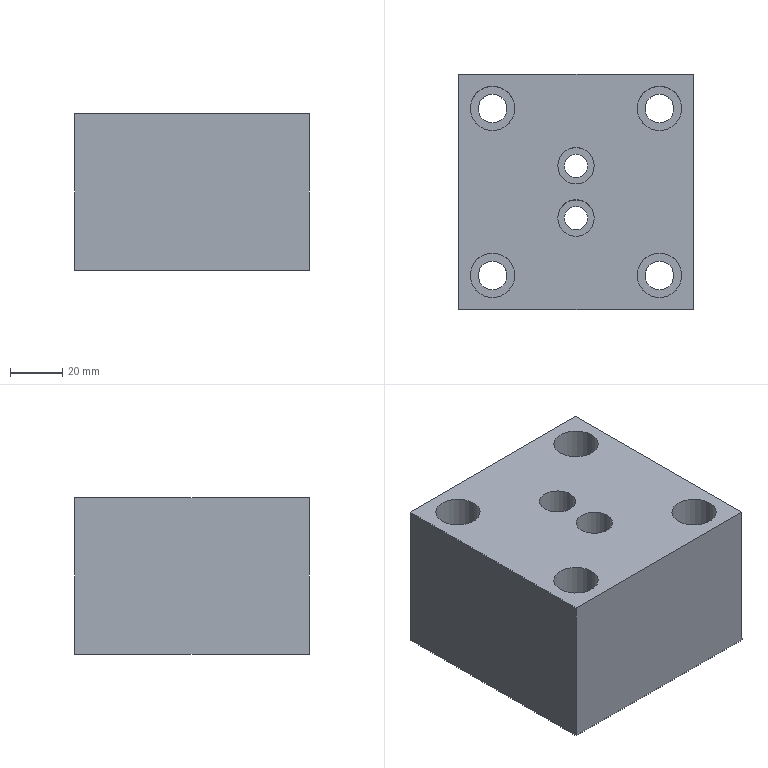Part | STEP file | PN_0003_id1490_x_t | 1 solid | 24 faces | box 90 x 90 x 60 mm | volume 430512 mm3 | plane 12 | cylinder 12 | commonest cylinder face diameters 11 x4 17 x4 9 x2 14 x2
STEP:
#1=CARTESIAN_POINT('',(-298.5,92.,155.));
#2=VERTEX_POINT('',#1);
#3=CARTESIAN_POINT('',(-293.,92.,155.));
#4=DIRECTION('',(0.,0.,1.));
#5=DIRECTION('',(-1.,0.,0.));
#6=AXIS2_PLACEMENT_3D('',#3,#4,#5);
#7=CIRCLE('',#6,5.5);
#8=EDGE_CURVE('',#2,#2,#7,.T.);
#9=ORIENTED_EDGE('',*,*,#8,.T.);
#10=EDGE_LOOP('',(#9));
#11=FACE_BOUND('',#10,.T.);
#12=CARTESIAN_POINT('',(-351.5,92.,155.));
#13=VERTEX_POINT('',#12);
#14=CARTESIAN_POINT('',(-357.,92.,155.));
#15=DIRECTION('',(0.,0.,-1.));
#16=DIRECTION('',(1.,0.,0.));
#17=AXIS2_PLACEMENT_3D('',#14,#15,#16);
#18=CIRCLE('',#17,5.5);
#19=EDGE_CURVE('',#13,#13,#18,.T.);
#20=ORIENTED_EDGE('',*,*,#19,.F.);
#21=EDGE_LOOP('',(#20));
#22=FACE_BOUND('',#21,.T.);
#23=CARTESIAN_POINT('',(-298.5,28.,155.));
#24=VERTEX_POINT('',#23);
#25=CARTESIAN_POINT('',(-293.,28.,155.));
#26=DIRECTION('',(0.,0.,-1.));
#27=DIRECTION('',(-1.,0.,0.));
#28=AXIS2_PLACEMENT_3D('',#25,#26,#27);
#29=CIRCLE('',#28,5.5);
#30=EDGE_CURVE('',#24,#24,#29,.T.);
#31=ORIENTED_EDGE('',*,*,#30,.F.);
#32=EDGE_LOOP('',(#31));
#33=FACE_BOUND('',#32,.T.);
#34=CARTESIAN_POINT('',(-351.5,28.,155.));
#35=VERTEX_POINT('',#34);
#36=CARTESIAN_POINT('',(-357.,28.,155.));
#37=DIRECTION('',(0.,0.,1.));
#38=DIRECTION('',(1.,0.,0.));
#39=AXIS2_PLACEMENT_3D('',#36,#37,#38);
#40=CIRCLE('',#39,5.5);
#41=EDGE_CURVE('',#35,#35,#40,.T.);
#42=ORIENTED_EDGE('',*,*,#41,.T.);
#43=EDGE_LOOP('',(#42));
#44=FACE_BOUND('',#43,.T.);
#45=CARTESIAN_POINT('',(-320.5,50.,155.));
#46=VERTEX_POINT('',#45);
#47=CARTESIAN_POINT('',(-325.,50.,155.));
#48=DIRECTION('',(0.,0.,1.));
#49=DIRECTION('',(1.,0.,0.));
#50=AXIS2_PLACEMENT_3D('',#47,#48,#49);
#51=CIRCLE('',#50,4.5);
#52=EDGE_CURVE('',#46,#46,#51,.T.);
#53=ORIENTED_EDGE('',*,*,#52,.T.);
#54=EDGE_LOOP('',(#53));
#55=FACE_BOUND('',#54,.T.);
#56=CARTESIAN_POINT('',(-320.5,70.,155.));
#57=VERTEX_POINT('',#56);
#58=CARTESIAN_POINT('',(-325.,70.,155.));
#59=DIRECTION('',(0.,0.,1.));
#60=DIRECTION('',(1.,0.,0.));
#61=AXIS2_PLACEMENT_3D('',#58,#59,#60);
#62=CIRCLE('',#61,4.5);
#63=EDGE_CURVE('',#57,#57,#62,.T.);
#64=ORIENTED_EDGE('',*,*,#63,.T.);
#65=EDGE_LOOP('',(#64));
#66=FACE_BOUND('',#65,.T.);
#67=CARTESIAN_POINT('',(-370.,15.,155.));
#68=VERTEX_POINT('',#67);
#69=CARTESIAN_POINT('',(-280.,15.,155.));
#70=VERTEX_POINT('',#69);
#71=CARTESIAN_POINT('',(-325.,15.,155.));
#72=DIRECTION('',(1.,0.,0.));
#73=VECTOR('',#72,1.);
#74=LINE('',#71,#73);
#75=EDGE_CURVE('',#68,#70,#74,.T.);
#76=ORIENTED_EDGE('',*,*,#75,.F.);
#77=CARTESIAN_POINT('',(-370.,105.,155.));
#78=VERTEX_POINT('',#77);
#79=CARTESIAN_POINT('',(-370.,-7.4,155.));
#80=DIRECTION('',(0.,-1.,0.));
#81=VECTOR('',#80,1.);
#82=LINE('',#79,#81);
#83=EDGE_CURVE('',#78,#68,#82,.T.);
#84=ORIENTED_EDGE('',*,*,#83,.F.);
#85=CARTESIAN_POINT('',(-280.,105.,155.));
#86=VERTEX_POINT('',#85);
#87=CARTESIAN_POINT('',(-325.,105.,155.));
#88=DIRECTION('',(-1.,0.,0.));
#89=VECTOR('',#88,1.);
#90=LINE('',#87,#89);
#91=EDGE_CURVE('',#86,#78,#90,.T.);
#92=ORIENTED_EDGE('',*,*,#91,.F.);
#93=CARTESIAN_POINT('',(-280.,60.,155.));
#94=DIRECTION('',(0.,1.,0.));
#95=VECTOR('',#94,1.);
#96=LINE('',#93,#95);
#97=EDGE_CURVE('',#70,#86,#96,.T.);
#98=ORIENTED_EDGE('',*,*,#97,.F.);
#99=EDGE_LOOP('',(#76,#84,#92,#98));
#100=FACE_BOUND('',#99,.T.);
#101=CARTESIAN_POINT('',(88.5,-1.,155.));
#102=DIRECTION('',(0.,0.,-1.));
#103=DIRECTION('',(1.,0.,0.));
#104=AXIS2_PLACEMENT_3D('',#101,#102,#103);
#105=PLANE('',#104);
#106=ADVANCED_FACE('',(#11,#22,#33,#44,#55,#66,#100),#105,.T.);
#107=CARTESIAN_POINT('',(-370.,15.,215.));
#108=VERTEX_POINT('',#107);
#109=CARTESIAN_POINT('',(-370.,15.,155.));
#110=DIRECTION('',(0.,0.,-1.));
#111=VECTOR('',#110,1.);
#112=LINE('',#109,#111);
#113=EDGE_CURVE('',#108,#68,#112,.T.);
#114=ORIENTED_EDGE('',*,*,#113,.T.);
#115=ORIENTED_EDGE('',*,*,#75,.T.);
#116=CARTESIAN_POINT('',(-280.,15.,215.));
#117=VERTEX_POINT('',#116);
#118=CARTESIAN_POINT('',(-280.,15.,155.));
#119=DIRECTION('',(0.,0.,-1.));
#120=VECTOR('',#119,1.);
#121=LINE('',#118,#120);
#122=EDGE_CURVE('',#117,#70,#121,.T.);
#123=ORIENTED_EDGE('',*,*,#122,.F.);
#124=CARTESIAN_POINT('',(-325.,15.,215.));
#125=DIRECTION('',(-1.,0.,0.));
#126=VECTOR('',#125,1.);
#127=LINE('',#124,#126);
#128=EDGE_CURVE('',#117,#108,#127,.T.);
#129=ORIENTED_EDGE('',*,*,#128,.T.);
#130=EDGE_LOOP('',(#114,#115,#123,#129));
#131=FACE_OUTER_BOUND('',#130,.T.);
#132=CARTESIAN_POINT('',(-325.,15.,155.));
#133=DIRECTION('',(0.,-1.,0.));
#134=DIRECTION('',(0.,0.,-1.));
#135=AXIS2_PLACEMENT_3D('',#132,#133,#134);
#136=PLANE('',#135);
#137=ADVANCED_FACE('',(#131),#136,.T.);
#138=ORIENTED_EDGE('',*,*,#122,.T.);
#139=ORIENTED_EDGE('',*,*,#97,.T.);
#140=CARTESIAN_POINT('',(-280.,105.,215.));
#141=VERTEX_POINT('',#140);
#142=CARTESIAN_POINT('',(-280.,105.,155.));
#143=DIRECTION('',(0.,0.,-1.));
#144=VECTOR('',#143,1.);
#145=LINE('',#142,#144);
#146=EDGE_CURVE('',#141,#86,#145,.T.);
#147=ORIENTED_EDGE('',*,*,#146,.F.);
#148=CARTESIAN_POINT('',(-280.,60.,215.));
#149=DIRECTION('',(0.,-1.,0.));
#150=VECTOR('',#149,1.);
#151=LINE('',#148,#150);
#152=EDGE_CURVE('',#141,#117,#151,.T.);
#153=ORIENTED_EDGE('',*,*,#152,.T.);
#154=EDGE_LOOP('',(#138,#139,#147,#153));
#155=FACE_OUTER_BOUND('',#154,.T.);
#156=CARTESIAN_POINT('',(-280.,60.,155.));
#157=DIRECTION('',(1.,0.,0.));
#158=DIRECTION('',(0.,0.,-1.));
#159=AXIS2_PLACEMENT_3D('',#156,#157,#158);
#160=PLANE('',#159);
#161=ADVANCED_FACE('',(#155),#160,.T.);
#162=ORIENTED_EDGE('',*,*,#146,.T.);
#163=ORIENTED_EDGE('',*,*,#91,.T.);
#164=CARTESIAN_POINT('',(-370.,105.,215.));
#165=VERTEX_POINT('',#164);
#166=CARTESIAN_POINT('',(-370.,105.,138.004));
#167=DIRECTION('',(0.,0.,-1.));
#168=VECTOR('',#167,1.);
#169=LINE('',#166,#168);
#170=EDGE_CURVE('',#165,#78,#169,.T.);
#171=ORIENTED_EDGE('',*,*,#170,.F.);
#172=CARTESIAN_POINT('',(-325.,105.,215.));
#173=DIRECTION('',(1.,0.,0.));
#174=VECTOR('',#173,1.);
#175=LINE('',#172,#174);
#176=EDGE_CURVE('',#165,#141,#175,.T.);
#177=ORIENTED_EDGE('',*,*,#176,.T.);
#178=EDGE_LOOP('',(#162,#163,#171,#177));
#179=FACE_OUTER_BOUND('',#178,.T.);
#180=CARTESIAN_POINT('',(-325.,105.,155.));
#181=DIRECTION('',(0.,1.,0.));
#182=DIRECTION('',(0.,0.,1.));
#183=AXIS2_PLACEMENT_3D('',#180,#181,#182);
#184=PLANE('',#183);
#185=ADVANCED_FACE('',(#179),#184,.T.);
#186=CARTESIAN_POINT('',(-284.5,92.,215.));
#187=VERTEX_POINT('',#186);
#188=CARTESIAN_POINT('',(-293.,92.,215.));
#189=DIRECTION('',(0.,0.,-1.));
#190=DIRECTION('',(1.,0.,0.));
#191=AXIS2_PLACEMENT_3D('',#188,#189,#190);
#192=CIRCLE('',#191,8.5);
#193=EDGE_CURVE('',#187,#187,#192,.T.);
#194=ORIENTED_EDGE('',*,*,#193,.T.);
#195=EDGE_LOOP('',(#194));
#196=FACE_BOUND('',#195,.T.);
#197=CARTESIAN_POINT('',(-365.5,92.,215.));
#198=VERTEX_POINT('',#197);
#199=CARTESIAN_POINT('',(-357.,92.,215.));
#200=DIRECTION('',(0.,0.,1.));
#201=DIRECTION('',(-1.,0.,0.));
#202=AXIS2_PLACEMENT_3D('',#199,#200,#201);
#203=CIRCLE('',#202,8.5);
#204=EDGE_CURVE('',#198,#198,#203,.T.);
#205=ORIENTED_EDGE('',*,*,#204,.F.);
#206=EDGE_LOOP('',(#205));
#207=FACE_BOUND('',#206,.T.);
#208=CARTESIAN_POINT('',(-284.5,28.,215.));
#209=VERTEX_POINT('',#208);
#210=CARTESIAN_POINT('',(-293.,28.,215.));
#211=DIRECTION('',(0.,0.,1.));
#212=DIRECTION('',(1.,0.,0.));
#213=AXIS2_PLACEMENT_3D('',#210,#211,#212);
#214=CIRCLE('',#213,8.5);
#215=EDGE_CURVE('',#209,#209,#214,.T.);
#216=ORIENTED_EDGE('',*,*,#215,.F.);
#217=EDGE_LOOP('',(#216));
#218=FACE_BOUND('',#217,.T.);
#219=CARTESIAN_POINT('',(-365.5,28.,215.));
#220=VERTEX_POINT('',#219);
#221=CARTESIAN_POINT('',(-357.,28.,215.));
#222=DIRECTION('',(0.,0.,-1.));
#223=DIRECTION('',(-1.,0.,0.));
#224=AXIS2_PLACEMENT_3D('',#221,#222,#223);
#225=CIRCLE('',#224,8.5);
#226=EDGE_CURVE('',#220,#220,#225,.T.);
#227=ORIENTED_EDGE('',*,*,#226,.T.);
#228=EDGE_LOOP('',(#227));
#229=FACE_BOUND('',#228,.T.);
#230=CARTESIAN_POINT('',(-332.,50.,215.));
#231=VERTEX_POINT('',#230);
#232=CARTESIAN_POINT('',(-325.,50.,215.));
#233=DIRECTION('',(0.,0.,-1.));
#234=DIRECTION('',(-1.,0.,0.));
#235=AXIS2_PLACEMENT_3D('',#232,#233,#234);
#236=CIRCLE('',#235,7.);
#237=EDGE_CURVE('',#231,#231,#236,.T.);
#238=ORIENTED_EDGE('',*,*,#237,.T.);
#239=EDGE_LOOP('',(#238));
#240=FACE_BOUND('',#239,.T.);
#241=CARTESIAN_POINT('',(-332.,70.,215.));
#242=VERTEX_POINT('',#241);
#243=CARTESIAN_POINT('',(-325.,70.,215.));
#244=DIRECTION('',(0.,0.,-1.));
#245=DIRECTION('',(-1.,0.,0.));
#246=AXIS2_PLACEMENT_3D('',#243,#244,#245);
#247=CIRCLE('',#246,7.);
#248=EDGE_CURVE('',#242,#242,#247,.T.);
#249=ORIENTED_EDGE('',*,*,#248,.T.);
#250=EDGE_LOOP('',(#249));
#251=FACE_BOUND('',#250,.T.);
#252=CARTESIAN_POINT('',(-370.,-7.4,215.));
#253=DIRECTION('',(0.,1.,0.));
#254=VECTOR('',#253,1.);
#255=LINE('',#252,#254);
#256=EDGE_CURVE('',#108,#165,#255,.T.);
#257=ORIENTED_EDGE('',*,*,#256,.F.);
#258=ORIENTED_EDGE('',*,*,#128,.F.);
#259=ORIENTED_EDGE('',*,*,#152,.F.);
#260=ORIENTED_EDGE('',*,*,#176,.F.);
#261=EDGE_LOOP('',(#257,#258,#259,#260));
#262=FACE_BOUND('',#261,.T.);
#263=CARTESIAN_POINT('',(133.5,-1.,215.));
#264=DIRECTION('',(0.,0.,-1.));
#265=DIRECTION('',(1.,0.,0.));
#266=AXIS2_PLACEMENT_3D('',#263,#264,#265);
#267=PLANE('',#266);
#268=ADVANCED_FACE('',(#196,#207,#218,#229,#240,#251,#262),#267,.F.);
#269=ORIENTED_EDGE('',*,*,#256,.T.);
#270=ORIENTED_EDGE('',*,*,#170,.T.);
#271=ORIENTED_EDGE('',*,*,#83,.T.);
#272=ORIENTED_EDGE('',*,*,#113,.F.);
#273=EDGE_LOOP('',(#269,#270,#271,#272));
#274=FACE_OUTER_BOUND('',#273,.T.);
#275=CARTESIAN_POINT('',(-370.,-7.4,138.004));
#276=DIRECTION('',(-1.,0.,0.));
#277=DIRECTION('',(0.,0.,-1.));
#278=AXIS2_PLACEMENT_3D('',#275,#276,#277);
#279=PLANE('',#278);
#280=ADVANCED_FACE('',(#274),#279,.T.);
#281=CARTESIAN_POINT('',(-329.5,70.,164.));
#282=VERTEX_POINT('',#281);
#283=CARTESIAN_POINT('',(-325.,70.,164.));
#284=DIRECTION('',(0.,0.,-1.));
#285=DIRECTION('',(-1.,0.,0.));
#286=AXIS2_PLACEMENT_3D('',#283,#284,#285);
#287=CIRCLE('',#286,4.5);
#288=EDGE_CURVE('',#282,#282,#287,.T.);
#289=ORIENTED_EDGE('',*,*,#288,.F.);
#290=EDGE_LOOP('',(#289));
#291=FACE_BOUND('',#290,.T.);
#292=ORIENTED_EDGE('',*,*,#63,.F.);
#293=EDGE_LOOP('',(#292));
#294=FACE_BOUND('',#293,.T.);
#295=CARTESIAN_POINT('',(-325.,70.,155.));
#296=DIRECTION('',(0.,0.,1.));
#297=DIRECTION('',(1.,0.,0.));
#298=AXIS2_PLACEMENT_3D('',#295,#296,#297);
#299=CYLINDRICAL_SURFACE('',#298,4.5);
#300=ADVANCED_FACE('',(#291,#294),#299,.F.);
#301=ORIENTED_EDGE('',*,*,#288,.T.);
#302=EDGE_LOOP('',(#301));
#303=FACE_BOUND('',#302,.T.);
#304=CARTESIAN_POINT('',(-318.,70.,164.));
#305=VERTEX_POINT('',#304);
#306=CARTESIAN_POINT('',(-325.,70.,164.));
#307=DIRECTION('',(0.,0.,-1.));
#308=DIRECTION('',(1.,0.,0.));
#309=AXIS2_PLACEMENT_3D('',#306,#307,#308);
#310=CIRCLE('',#309,7.);
#311=EDGE_CURVE('',#305,#305,#310,.T.);
#312=ORIENTED_EDGE('',*,*,#311,.F.);
#313=EDGE_LOOP('',(#312));
#314=FACE_BOUND('',#313,.T.);
#315=CARTESIAN_POINT('',(-325.,70.,164.));
#316=DIRECTION('',(0.,0.,-1.));
#317=DIRECTION('',(-1.,0.,0.));
#318=AXIS2_PLACEMENT_3D('',#315,#316,#317);
#319=PLANE('',#318);
#320=ADVANCED_FACE('',(#303,#314),#319,.F.);
#321=ORIENTED_EDGE('',*,*,#248,.F.);
#322=EDGE_LOOP('',(#321));
#323=FACE_BOUND('',#322,.T.);
#324=ORIENTED_EDGE('',*,*,#311,.T.);
#325=EDGE_LOOP('',(#324));
#326=FACE_BOUND('',#325,.T.);
#327=CARTESIAN_POINT('',(-325.,70.,164.));
#328=DIRECTION('',(0.,0.,1.));
#329=DIRECTION('',(1.,0.,0.));
#330=AXIS2_PLACEMENT_3D('',#327,#328,#329);
#331=CYLINDRICAL_SURFACE('',#330,7.);
#332=ADVANCED_FACE('',(#323,#326),#331,.F.);
#333=CARTESIAN_POINT('',(-329.5,50.,164.));
#334=VERTEX_POINT('',#333);
#335=CARTESIAN_POINT('',(-325.,50.,164.));
#336=DIRECTION('',(0.,0.,-1.));
#337=DIRECTION('',(-1.,0.,0.));
#338=AXIS2_PLACEMENT_3D('',#335,#336,#337);
#339=CIRCLE('',#338,4.5);
#340=EDGE_CURVE('',#334,#334,#339,.T.);
#341=ORIENTED_EDGE('',*,*,#340,.F.);
#342=EDGE_LOOP('',(#341));
#343=FACE_BOUND('',#342,.T.);
#344=ORIENTED_EDGE('',*,*,#52,.F.);
#345=EDGE_LOOP('',(#344));
#346=FACE_BOUND('',#345,.T.);
#347=CARTESIAN_POINT('',(-325.,50.,155.));
#348=DIRECTION('',(0.,0.,1.));
#349=DIRECTION('',(1.,0.,0.));
#350=AXIS2_PLACEMENT_3D('',#347,#348,#349);
#351=CYLINDRICAL_SURFACE('',#350,4.5);
#352=ADVANCED_FACE('',(#343,#346),#351,.F.);
#353=ORIENTED_EDGE('',*,*,#340,.T.);
#354=EDGE_LOOP('',(#353));
#355=FACE_BOUND('',#354,.T.);
#356=CARTESIAN_POINT('',(-318.,50.,164.));
#357=VERTEX_POINT('',#356);
#358=CARTESIAN_POINT('',(-325.,50.,164.));
#359=DIRECTION('',(0.,0.,-1.));
#360=DIRECTION('',(1.,0.,0.));
#361=AXIS2_PLACEMENT_3D('',#358,#359,#360);
#362=CIRCLE('',#361,7.);
#363=EDGE_CURVE('',#357,#357,#362,.T.);
#364=ORIENTED_EDGE('',*,*,#363,.F.);
#365=EDGE_LOOP('',(#364));
#366=FACE_BOUND('',#365,.T.);
#367=CARTESIAN_POINT('',(-325.,50.,164.));
#368=DIRECTION('',(0.,0.,-1.));
#369=DIRECTION('',(-1.,0.,0.));
#370=AXIS2_PLACEMENT_3D('',#367,#368,#369);
#371=PLANE('',#370);
#372=ADVANCED_FACE('',(#355,#366),#371,.F.);
#373=ORIENTED_EDGE('',*,*,#237,.F.);
#374=EDGE_LOOP('',(#373));
#375=FACE_BOUND('',#374,.T.);
#376=ORIENTED_EDGE('',*,*,#363,.T.);
#377=EDGE_LOOP('',(#376));
#378=FACE_BOUND('',#377,.T.);
#379=CARTESIAN_POINT('',(-325.,50.,164.));
#380=DIRECTION('',(0.,0.,1.));
#381=DIRECTION('',(1.,0.,0.));
#382=AXIS2_PLACEMENT_3D('',#379,#380,#381);
#383=CYLINDRICAL_SURFACE('',#382,7.);
#384=ADVANCED_FACE('',(#375,#378),#383,.F.);
#385=CARTESIAN_POINT('',(-362.5,28.,185.));
#386=VERTEX_POINT('',#385);
#387=CARTESIAN_POINT('',(-357.,28.,185.));
#388=DIRECTION('',(0.,0.,-1.));
#389=DIRECTION('',(-1.,0.,0.));
#390=AXIS2_PLACEMENT_3D('',#387,#388,#389);
#391=CIRCLE('',#390,5.5);
#392=EDGE_CURVE('',#386,#386,#391,.T.);
#393=ORIENTED_EDGE('',*,*,#392,.F.);
#394=EDGE_LOOP('',(#393));
#395=FACE_BOUND('',#394,.T.);
#396=ORIENTED_EDGE('',*,*,#41,.F.);
#397=EDGE_LOOP('',(#396));
#398=FACE_BOUND('',#397,.T.);
#399=CARTESIAN_POINT('',(-357.,28.,155.));
#400=DIRECTION('',(0.,0.,1.));
#401=DIRECTION('',(1.,0.,0.));
#402=AXIS2_PLACEMENT_3D('',#399,#400,#401);
#403=CYLINDRICAL_SURFACE('',#402,5.5);
#404=ADVANCED_FACE('',(#395,#398),#403,.F.);
#405=ORIENTED_EDGE('',*,*,#392,.T.);
#406=EDGE_LOOP('',(#405));
#407=FACE_BOUND('',#406,.T.);
#408=CARTESIAN_POINT('',(-348.5,28.,185.));
#409=VERTEX_POINT('',#408);
#410=CARTESIAN_POINT('',(-357.,28.,185.));
#411=DIRECTION('',(0.,0.,-1.));
#412=DIRECTION('',(1.,0.,0.));
#413=AXIS2_PLACEMENT_3D('',#410,#411,#412);
#414=CIRCLE('',#413,8.5);
#415=EDGE_CURVE('',#409,#409,#414,.T.);
#416=ORIENTED_EDGE('',*,*,#415,.F.);
#417=EDGE_LOOP('',(#416));
#418=FACE_BOUND('',#417,.T.);
#419=CARTESIAN_POINT('',(-357.,28.,185.));
#420=DIRECTION('',(0.,0.,-1.));
#421=DIRECTION('',(-1.,0.,0.));
#422=AXIS2_PLACEMENT_3D('',#419,#420,#421);
#423=PLANE('',#422);
#424=ADVANCED_FACE('',(#407,#418),#423,.F.);
#425=ORIENTED_EDGE('',*,*,#226,.F.);
#426=EDGE_LOOP('',(#425));
#427=FACE_BOUND('',#426,.T.);
#428=ORIENTED_EDGE('',*,*,#415,.T.);
#429=EDGE_LOOP('',(#428));
#430=FACE_BOUND('',#429,.T.);
#431=CARTESIAN_POINT('',(-357.,28.,185.));
#432=DIRECTION('',(0.,0.,1.));
#433=DIRECTION('',(1.,0.,0.));
#434=AXIS2_PLACEMENT_3D('',#431,#432,#433);
#435=CYLINDRICAL_SURFACE('',#434,8.5);
#436=ADVANCED_FACE('',(#427,#430),#435,.F.);
#437=CARTESIAN_POINT('',(-287.5,28.,185.));
#438=VERTEX_POINT('',#437);
#439=CARTESIAN_POINT('',(-293.,28.,185.));
#440=DIRECTION('',(0.,0.,1.));
#441=DIRECTION('',(1.,0.,0.));
#442=AXIS2_PLACEMENT_3D('',#439,#440,#441);
#443=CIRCLE('',#442,5.5);
#444=EDGE_CURVE('',#438,#438,#443,.T.);
#445=ORIENTED_EDGE('',*,*,#444,.T.);
#446=EDGE_LOOP('',(#445));
#447=FACE_BOUND('',#446,.T.);
#448=ORIENTED_EDGE('',*,*,#30,.T.);
#449=EDGE_LOOP('',(#448));
#450=FACE_BOUND('',#449,.T.);
#451=CARTESIAN_POINT('',(-293.,28.,155.));
#452=DIRECTION('',(0.,0.,1.));
#453=DIRECTION('',(-1.,0.,0.));
#454=AXIS2_PLACEMENT_3D('',#451,#452,#453);
#455=CYLINDRICAL_SURFACE('',#454,5.5);
#456=ADVANCED_FACE('',(#447,#450),#455,.F.);
#457=ORIENTED_EDGE('',*,*,#444,.F.);
#458=EDGE_LOOP('',(#457));
#459=FACE_BOUND('',#458,.T.);
#460=CARTESIAN_POINT('',(-301.5,28.,185.));
#461=VERTEX_POINT('',#460);
#462=CARTESIAN_POINT('',(-293.,28.,185.));
#463=DIRECTION('',(0.,0.,1.));
#464=DIRECTION('',(-1.,0.,0.));
#465=AXIS2_PLACEMENT_3D('',#462,#463,#464);
#466=CIRCLE('',#465,8.5);
#467=EDGE_CURVE('',#461,#461,#466,.T.);
#468=ORIENTED_EDGE('',*,*,#467,.T.);
#469=EDGE_LOOP('',(#468));
#470=FACE_BOUND('',#469,.T.);
#471=CARTESIAN_POINT('',(-293.,28.,185.));
#472=DIRECTION('',(0.,0.,-1.));
#473=DIRECTION('',(1.,0.,0.));
#474=AXIS2_PLACEMENT_3D('',#471,#472,#473);
#475=PLANE('',#474);
#476=ADVANCED_FACE('',(#459,#470),#475,.F.);
#477=ORIENTED_EDGE('',*,*,#215,.T.);
#478=EDGE_LOOP('',(#477));
#479=FACE_BOUND('',#478,.T.);
#480=ORIENTED_EDGE('',*,*,#467,.F.);
#481=EDGE_LOOP('',(#480));
#482=FACE_BOUND('',#481,.T.);
#483=CARTESIAN_POINT('',(-293.,28.,185.));
#484=DIRECTION('',(0.,0.,1.));
#485=DIRECTION('',(-1.,0.,0.));
#486=AXIS2_PLACEMENT_3D('',#483,#484,#485);
#487=CYLINDRICAL_SURFACE('',#486,8.5);
#488=ADVANCED_FACE('',(#479,#482),#487,.F.);
#489=CARTESIAN_POINT('',(-362.5,92.,185.));
#490=VERTEX_POINT('',#489);
#491=CARTESIAN_POINT('',(-357.,92.,185.));
#492=DIRECTION('',(0.,0.,1.));
#493=DIRECTION('',(-1.,0.,0.));
#494=AXIS2_PLACEMENT_3D('',#491,#492,#493);
#495=CIRCLE('',#494,5.5);
#496=EDGE_CURVE('',#490,#490,#495,.T.);
#497=ORIENTED_EDGE('',*,*,#496,.T.);
#498=EDGE_LOOP('',(#497));
#499=FACE_BOUND('',#498,.T.);
#500=ORIENTED_EDGE('',*,*,#19,.T.);
#501=EDGE_LOOP('',(#500));
#502=FACE_BOUND('',#501,.T.);
#503=CARTESIAN_POINT('',(-357.,92.,155.));
#504=DIRECTION('',(0.,0.,1.));
#505=DIRECTION('',(1.,0.,0.));
#506=AXIS2_PLACEMENT_3D('',#503,#504,#505);
#507=CYLINDRICAL_SURFACE('',#506,5.5);
#508=ADVANCED_FACE('',(#499,#502),#507,.F.);
#509=ORIENTED_EDGE('',*,*,#496,.F.);
#510=EDGE_LOOP('',(#509));
#511=FACE_BOUND('',#510,.T.);
#512=CARTESIAN_POINT('',(-348.5,92.,185.));
#513=VERTEX_POINT('',#512);
#514=CARTESIAN_POINT('',(-357.,92.,185.));
#515=DIRECTION('',(0.,0.,1.));
#516=DIRECTION('',(1.,0.,0.));
#517=AXIS2_PLACEMENT_3D('',#514,#515,#516);
#518=CIRCLE('',#517,8.5);
#519=EDGE_CURVE('',#513,#513,#518,.T.);
#520=ORIENTED_EDGE('',*,*,#519,.T.);
#521=EDGE_LOOP('',(#520));
#522=FACE_BOUND('',#521,.T.);
#523=CARTESIAN_POINT('',(-357.,92.,185.));
#524=DIRECTION('',(0.,0.,-1.));
#525=DIRECTION('',(-1.,0.,0.));
#526=AXIS2_PLACEMENT_3D('',#523,#524,#525);
#527=PLANE('',#526);
#528=ADVANCED_FACE('',(#511,#522),#527,.F.);
#529=ORIENTED_EDGE('',*,*,#204,.T.);
#530=EDGE_LOOP('',(#529));
#531=FACE_BOUND('',#530,.T.);
#532=ORIENTED_EDGE('',*,*,#519,.F.);
#533=EDGE_LOOP('',(#532));
#534=FACE_BOUND('',#533,.T.);
#535=CARTESIAN_POINT('',(-357.,92.,185.));
#536=DIRECTION('',(0.,0.,1.));
#537=DIRECTION('',(1.,0.,0.));
#538=AXIS2_PLACEMENT_3D('',#535,#536,#537);
#539=CYLINDRICAL_SURFACE('',#538,8.5);
#540=ADVANCED_FACE('',(#531,#534),#539,.F.);
#541=CARTESIAN_POINT('',(-287.5,92.,185.));
#542=VERTEX_POINT('',#541);
#543=CARTESIAN_POINT('',(-293.,92.,185.));
#544=DIRECTION('',(0.,0.,-1.));
#545=DIRECTION('',(1.,0.,0.));
#546=AXIS2_PLACEMENT_3D('',#543,#544,#545);
#547=CIRCLE('',#546,5.5);
#548=EDGE_CURVE('',#542,#542,#547,.T.);
#549=ORIENTED_EDGE('',*,*,#548,.F.);
#550=EDGE_LOOP('',(#549));
#551=FACE_BOUND('',#550,.T.);
#552=ORIENTED_EDGE('',*,*,#8,.F.);
#553=EDGE_LOOP('',(#552));
#554=FACE_BOUND('',#553,.T.);
#555=CARTESIAN_POINT('',(-293.,92.,155.));
#556=DIRECTION('',(0.,0.,1.));
#557=DIRECTION('',(-1.,0.,0.));
#558=AXIS2_PLACEMENT_3D('',#555,#556,#557);
#559=CYLINDRICAL_SURFACE('',#558,5.5);
#560=ADVANCED_FACE('',(#551,#554),#559,.F.);
#561=ORIENTED_EDGE('',*,*,#548,.T.);
#562=EDGE_LOOP('',(#561));
#563=FACE_BOUND('',#562,.T.);
#564=CARTESIAN_POINT('',(-301.5,92.,185.));
#565=VERTEX_POINT('',#564);
#566=CARTESIAN_POINT('',(-293.,92.,185.));
#567=DIRECTION('',(0.,0.,-1.));
#568=DIRECTION('',(-1.,0.,0.));
#569=AXIS2_PLACEMENT_3D('',#566,#567,#568);
#570=CIRCLE('',#569,8.5);
#571=EDGE_CURVE('',#565,#565,#570,.T.);
#572=ORIENTED_EDGE('',*,*,#571,.F.);
#573=EDGE_LOOP('',(#572));
#574=FACE_BOUND('',#573,.T.);
#575=CARTESIAN_POINT('',(-293.,92.,185.));
#576=DIRECTION('',(0.,0.,-1.));
#577=DIRECTION('',(1.,0.,0.));
#578=AXIS2_PLACEMENT_3D('',#575,#576,#577);
#579=PLANE('',#578);
#580=ADVANCED_FACE('',(#563,#574),#579,.F.);
#581=ORIENTED_EDGE('',*,*,#193,.F.);
#582=EDGE_LOOP('',(#581));
#583=FACE_BOUND('',#582,.T.);
#584=ORIENTED_EDGE('',*,*,#571,.T.);
#585=EDGE_LOOP('',(#584));
#586=FACE_BOUND('',#585,.T.);
#587=CARTESIAN_POINT('',(-293.,92.,185.));
#588=DIRECTION('',(0.,0.,1.));
#589=DIRECTION('',(-1.,0.,0.));
#590=AXIS2_PLACEMENT_3D('',#587,#588,#589);
#591=CYLINDRICAL_SURFACE('',#590,8.5);
#592=ADVANCED_FACE('',(#583,#586),#591,.F.);
#593=CLOSED_SHELL('',(#106,#137,#161,#185,#268,#280,#300,#320,#332,#352,#372,#384,#404,#424,#436,#456,#476,#488,#508,#528,#540,#560,#580,#592));
#594=MANIFOLD_SOLID_BREP('',#593);
#595=(LENGTH_UNIT()NAMED_UNIT(*)SI_UNIT(.MILLI.,.METRE.));
#596=UNCERTAINTY_MEASURE_WITH_UNIT(LENGTH_MEASURE(0.00002),#595,'','');
#597=(NAMED_UNIT(*)PLANE_ANGLE_UNIT()SI_UNIT($,.RADIAN.));
#598=PLANE_ANGLE_MEASURE_WITH_UNIT(PLANE_ANGLE_MEASURE(0.01745),#597);
#599=DIMENSIONAL_EXPONENTS(0.,0.,0.,0.,0.,0.,0.);
#600=(CONVERSION_BASED_UNIT('DEGREE',#598)NAMED_UNIT(#599)PLANE_ANGLE_UNIT());
#601=(NAMED_UNIT(*)SI_UNIT($,.STERADIAN.)SOLID_ANGLE_UNIT());
#602=(GEOMETRIC_REPRESENTATION_CONTEXT(3)GLOBAL_UNCERTAINTY_ASSIGNED_CONTEXT((#596))GLOBAL_UNIT_ASSIGNED_CONTEXT((#595,#600,#601))REPRESENTATION_CONTEXT('',''));
#603=ADVANCED_BREP_SHAPE_REPRESENTATION('',(#594),#602);